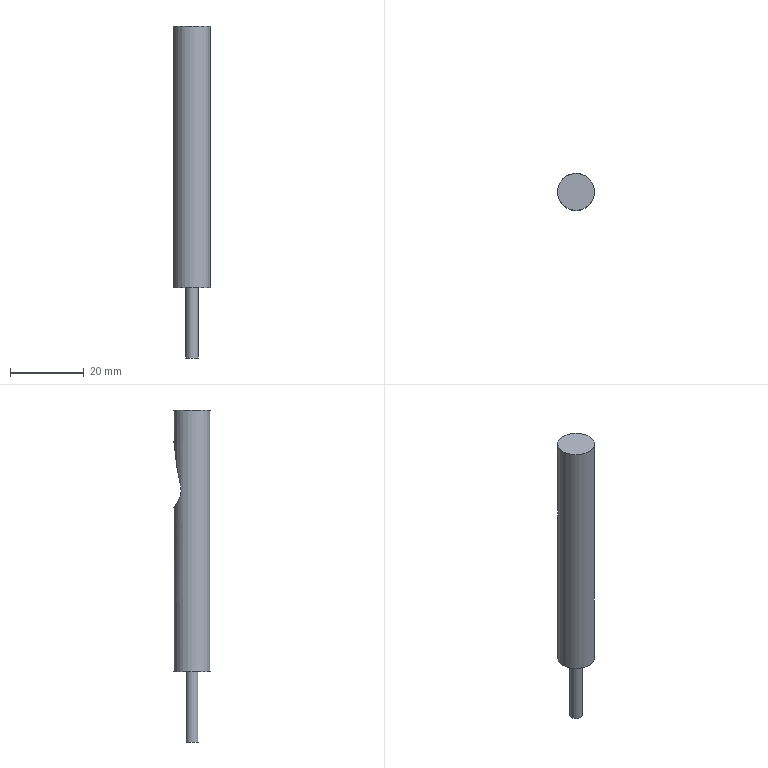Part | NX | features solid 2 | 1 solid | 8 faces | volume 5491 mm3 | plane 3 | cylinder 2 | sphere 2 | cone 1 | commonest cylinder face diameters 3.3 x1 10 x1
STEP:
#1=CARTESIAN_POINT('',(299.146,-146.033,62.125));
#2=VERTEX_POINT('',#1);
#3=CARTESIAN_POINT('',(296.661,-144.346,73.375));
#4=VERTEX_POINT('',#3);
#5=CARTESIAN_POINT('',(299.146,-146.033,62.125));
#6=CARTESIAN_POINT('',(298.481,-145.193,65.863));
#7=CARTESIAN_POINT('',(297.602,-144.628,69.613));
#8=CARTESIAN_POINT('',(296.661,-144.346,73.375));
#9=B_SPLINE_CURVE_WITH_KNOTS('',3,(#5,#6,#7,#8),.UNSPECIFIED.,.F.,.F.,(4,4),(0.000000208,0.01165),.UNSPECIFIED.);
#10=EDGE_CURVE('',#2,#4,#9,.T.);
#11=ORIENTED_EDGE('',*,*,#10,.T.);
#12=CARTESIAN_POINT('',(293.787,-144.346,73.375));
#13=VERTEX_POINT('',#12);
#14=CARTESIAN_POINT('',(296.661,-144.346,73.375));
#15=CARTESIAN_POINT('',(296.5,-144.298,74.02));
#16=CARTESIAN_POINT('',(295.226,-143.972,74.98));
#17=CARTESIAN_POINT('',(293.949,-144.298,74.02));
#18=CARTESIAN_POINT('',(293.787,-144.346,73.375));
#19=B_SPLINE_CURVE_WITH_KNOTS('',3,(#14,#15,#16,#17,#18),.UNSPECIFIED.,.F.,.F.,(4,1,4),(0.000000204,0.001971,0.003941),.UNSPECIFIED.);
#20=EDGE_CURVE('',#4,#13,#19,.T.);
#21=ORIENTED_EDGE('',*,*,#20,.T.);
#22=CARTESIAN_POINT('',(291.303,-146.033,62.125));
#23=VERTEX_POINT('',#22);
#24=CARTESIAN_POINT('',(293.787,-144.346,73.375));
#25=CARTESIAN_POINT('',(292.847,-144.628,69.611));
#26=CARTESIAN_POINT('',(291.968,-145.192,65.865));
#27=CARTESIAN_POINT('',(291.303,-146.033,62.125));
#28=B_SPLINE_CURVE_WITH_KNOTS('',3,(#24,#25,#26,#27),.UNSPECIFIED.,.F.,.F.,(4,4),(0.000000207,0.01167),.UNSPECIFIED.);
#29=EDGE_CURVE('',#13,#23,#28,.T.);
#30=ORIENTED_EDGE('',*,*,#29,.T.);
#31=CARTESIAN_POINT('',(291.303,-146.033,62.125));
#32=CARTESIAN_POINT('',(291.183,-146.184,61.454));
#33=CARTESIAN_POINT('',(291.164,-146.211,60.034));
#34=CARTESIAN_POINT('',(291.777,-145.43,58.139));
#35=CARTESIAN_POINT('',(293.154,-144.449,56.833));
#36=CARTESIAN_POINT('',(295.21,-143.98,56.336));
#37=CARTESIAN_POINT('',(297.287,-144.442,56.825));
#38=CARTESIAN_POINT('',(298.672,-145.43,58.139));
#39=CARTESIAN_POINT('',(299.284,-146.209,60.026));
#40=CARTESIAN_POINT('',(299.266,-146.185,61.453));
#41=CARTESIAN_POINT('',(299.146,-146.033,62.125));
#42=B_SPLINE_CURVE_WITH_KNOTS('',3,(#31,#32,#33,#34,#35,#36,#37,#38,#39,#40,#41),.UNSPECIFIED.,.F.,.F.,(4,1,1,1,1,1,1,1,4),(0.000000205,0.002065,0.00413,0.006195,0.00826,0.01033,0.01239,0.01446,0.01652),.UNSPECIFIED.);
#43=EDGE_CURVE('',#23,#2,#42,.T.);
#44=ORIENTED_EDGE('',*,*,#43,.T.);
#45=EDGE_LOOP('',(#11,#21,#30,#44));
#46=FACE_BOUND('',#45,.T.);
#47=CARTESIAN_POINT('',(300.224,-149.135,83.));
#48=VERTEX_POINT('',#47);
#49=CARTESIAN_POINT('',(295.224,-149.135,83.));
#50=DIRECTION('',(0.,0.,1.));
#51=DIRECTION('',(1.,0.,0.));
#52=AXIS2_PLACEMENT_3D('',#49,#50,#51);
#53=CIRCLE('',#52,5.);
#54=EDGE_CURVE('',#48,#48,#53,.T.);
#55=ORIENTED_EDGE('',*,*,#54,.F.);
#56=EDGE_LOOP('',(#55));
#57=FACE_BOUND('',#56,.T.);
#58=CARTESIAN_POINT('',(300.224,-149.135,12.));
#59=VERTEX_POINT('',#58);
#60=CARTESIAN_POINT('',(295.224,-149.135,12.));
#61=DIRECTION('',(0.,0.,1.));
#62=DIRECTION('',(1.,0.,0.));
#63=AXIS2_PLACEMENT_3D('',#60,#61,#62);
#64=CIRCLE('',#63,5.);
#65=EDGE_CURVE('',#59,#59,#64,.T.);
#66=ORIENTED_EDGE('',*,*,#65,.T.);
#67=EDGE_LOOP('',(#66));
#68=FACE_BOUND('',#67,.T.);
#69=CARTESIAN_POINT('',(295.224,-149.135,83.));
#70=DIRECTION('',(0.,0.,-1.));
#71=DIRECTION('',(-1.,0.,0.));
#72=AXIS2_PLACEMENT_3D('',#69,#70,#71);
#73=CYLINDRICAL_SURFACE('',#72,5.);
#74=ADVANCED_FACE('',(#46,#57,#68),#73,.T.);
#75=ORIENTED_EDGE('',*,*,#54,.T.);
#76=EDGE_LOOP('',(#75));
#77=FACE_BOUND('',#76,.T.);
#78=CARTESIAN_POINT('',(295.224,-149.135,83.));
#79=DIRECTION('',(0.,0.,1.));
#80=DIRECTION('',(1.,0.,0.));
#81=AXIS2_PLACEMENT_3D('',#78,#79,#80);
#82=PLANE('',#81);
#83=ADVANCED_FACE('',(#77),#82,.T.);
#84=CARTESIAN_POINT('',(296.874,-149.135,12.));
#85=VERTEX_POINT('',#84);
#86=CARTESIAN_POINT('',(295.224,-149.135,12.));
#87=DIRECTION('',(0.,0.,1.));
#88=DIRECTION('',(1.,0.,0.));
#89=AXIS2_PLACEMENT_3D('',#86,#87,#88);
#90=CIRCLE('',#89,1.65);
#91=EDGE_CURVE('',#85,#85,#90,.T.);
#92=ORIENTED_EDGE('',*,*,#91,.T.);
#93=EDGE_LOOP('',(#92));
#94=FACE_BOUND('',#93,.T.);
#95=ORIENTED_EDGE('',*,*,#65,.F.);
#96=EDGE_LOOP('',(#95));
#97=FACE_BOUND('',#96,.T.);
#98=CARTESIAN_POINT('',(295.224,-149.135,12.));
#99=DIRECTION('',(0.,0.,1.));
#100=DIRECTION('',(1.,0.,0.));
#101=AXIS2_PLACEMENT_3D('',#98,#99,#100);
#102=PLANE('',#101);
#103=ADVANCED_FACE('',(#94,#97),#102,.F.);
#104=CARTESIAN_POINT('',(296.874,-149.135,-7.));
#105=VERTEX_POINT('',#104);
#106=CARTESIAN_POINT('',(295.224,-149.135,-7.));
#107=DIRECTION('',(0.,0.,1.));
#108=DIRECTION('',(1.,0.,0.));
#109=AXIS2_PLACEMENT_3D('',#106,#107,#108);
#110=CIRCLE('',#109,1.65);
#111=EDGE_CURVE('',#105,#105,#110,.T.);
#112=ORIENTED_EDGE('',*,*,#111,.T.);
#113=EDGE_LOOP('',(#112));
#114=FACE_BOUND('',#113,.T.);
#115=ORIENTED_EDGE('',*,*,#91,.F.);
#116=EDGE_LOOP('',(#115));
#117=FACE_BOUND('',#116,.T.);
#118=CARTESIAN_POINT('',(295.224,-149.135,-7.));
#119=DIRECTION('',(0.,0.,1.));
#120=DIRECTION('',(1.,0.,0.));
#121=AXIS2_PLACEMENT_3D('',#118,#119,#120);
#122=CYLINDRICAL_SURFACE('',#121,1.65);
#123=ADVANCED_FACE('',(#114,#117),#122,.T.);
#124=ORIENTED_EDGE('',*,*,#111,.F.);
#125=EDGE_LOOP('',(#124));
#126=FACE_BOUND('',#125,.T.);
#127=CARTESIAN_POINT('',(295.224,-149.135,-7.));
#128=DIRECTION('',(0.,0.,1.));
#129=DIRECTION('',(1.,0.,0.));
#130=AXIS2_PLACEMENT_3D('',#127,#128,#129);
#131=PLANE('',#130);
#132=ADVANCED_FACE('',(#126),#131,.F.);
#133=CARTESIAN_POINT('',(295.224,-144.135,62.125));
#134=DIRECTION('',(0.,0.,-1.));
#135=DIRECTION('',(-1.,0.,0.));
#136=AXIS2_PLACEMENT_3D('',#133,#134,#135);
#137=CIRCLE('',#136,4.357);
#138=EDGE_CURVE('',#2,#23,#137,.T.);
#139=ORIENTED_EDGE('',*,*,#138,.F.);
#140=ORIENTED_EDGE('',*,*,#43,.F.);
#141=EDGE_LOOP('',(#139,#140));
#142=FACE_BOUND('',#141,.T.);
#143=CARTESIAN_POINT('',(295.224,-144.135,61.));
#144=DIRECTION('',(0.,0.,-1.));
#145=DIRECTION('',(1.,0.,0.));
#146=AXIS2_PLACEMENT_3D('',#143,#144,#145);
#147=SPHERICAL_SURFACE('',#146,4.5);
#148=ADVANCED_FACE('',(#142),#147,.F.);
#149=CARTESIAN_POINT('',(295.224,-144.135,73.375));
#150=DIRECTION('',(0.,0.,-1.));
#151=DIRECTION('',(-1.,0.,0.));
#152=AXIS2_PLACEMENT_3D('',#149,#150,#151);
#153=CIRCLE('',#152,1.452);
#154=EDGE_CURVE('',#4,#13,#153,.T.);
#155=ORIENTED_EDGE('',*,*,#154,.F.);
#156=ORIENTED_EDGE('',*,*,#10,.F.);
#157=ORIENTED_EDGE('',*,*,#138,.T.);
#158=ORIENTED_EDGE('',*,*,#29,.F.);
#159=EDGE_LOOP('',(#155,#156,#157,#158));
#160=FACE_BOUND('',#159,.T.);
#161=CARTESIAN_POINT('',(295.224,-144.135,62.125));
#162=DIRECTION('',(0.,0.,-1.));
#163=DIRECTION('',(-1.,0.,0.));
#164=AXIS2_PLACEMENT_3D('',#161,#162,#163);
#165=CONICAL_SURFACE('',#164,4.357,0.2527);
#166=ADVANCED_FACE('',(#160),#165,.F.);
#167=ORIENTED_EDGE('',*,*,#154,.T.);
#168=ORIENTED_EDGE('',*,*,#20,.F.);
#169=EDGE_LOOP('',(#167,#168));
#170=FACE_BOUND('',#169,.T.);
#171=CARTESIAN_POINT('',(295.224,-144.135,73.));
#172=DIRECTION('',(0.,0.,-1.));
#173=DIRECTION('',(1.,0.,0.));
#174=AXIS2_PLACEMENT_3D('',#171,#172,#173);
#175=SPHERICAL_SURFACE('',#174,1.5);
#176=ADVANCED_FACE('',(#170),#175,.F.);
#177=CLOSED_SHELL('',(#74,#83,#103,#123,#132,#148,#166,#176));
#178=MANIFOLD_SOLID_BREP('',#177);
#179=(LENGTH_UNIT()NAMED_UNIT(*)SI_UNIT(.MILLI.,.METRE.));
#180=UNCERTAINTY_MEASURE_WITH_UNIT(LENGTH_MEASURE(0.0508),#179,'','');
#181=(NAMED_UNIT(*)PLANE_ANGLE_UNIT()SI_UNIT($,.RADIAN.));
#182=(NAMED_UNIT(*)SI_UNIT($,.STERADIAN.)SOLID_ANGLE_UNIT());
#183=(GEOMETRIC_REPRESENTATION_CONTEXT(3)GLOBAL_UNCERTAINTY_ASSIGNED_CONTEXT((#180))GLOBAL_UNIT_ASSIGNED_CONTEXT((#179,#181,#182))REPRESENTATION_CONTEXT('',''));
#184=ADVANCED_BREP_SHAPE_REPRESENTATION('',(#178),#183);